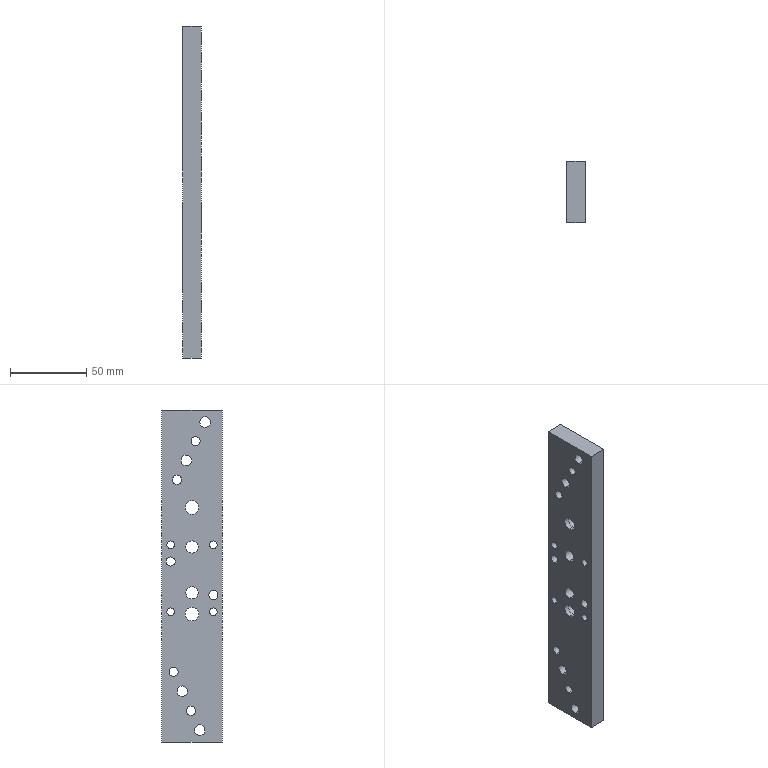Part | STEP file | OP10-152_side plate upper-L1 | 1 solid | 48 faces | box 12 x 40 x 218 mm | volume 95136 mm3 | cylinder 40 | plane 8 | commonest cylinder face diameters 6 x12 5 x8 7 x8 8 x4 9 x4 15 x4